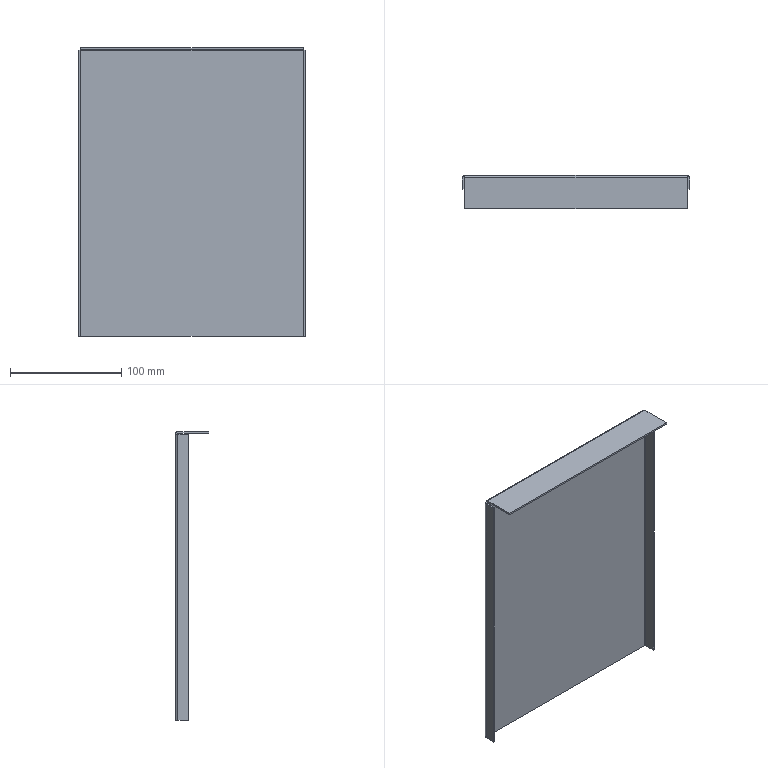Part | STEP file | A14-053 | 1 solid | 30 faces | box 204.473 x 29.929 x 260 mm | volume 95693 mm3 | plane 24 | cylinder 6 | commonest cylinder face diameters 1.473 x3 4.473 x3